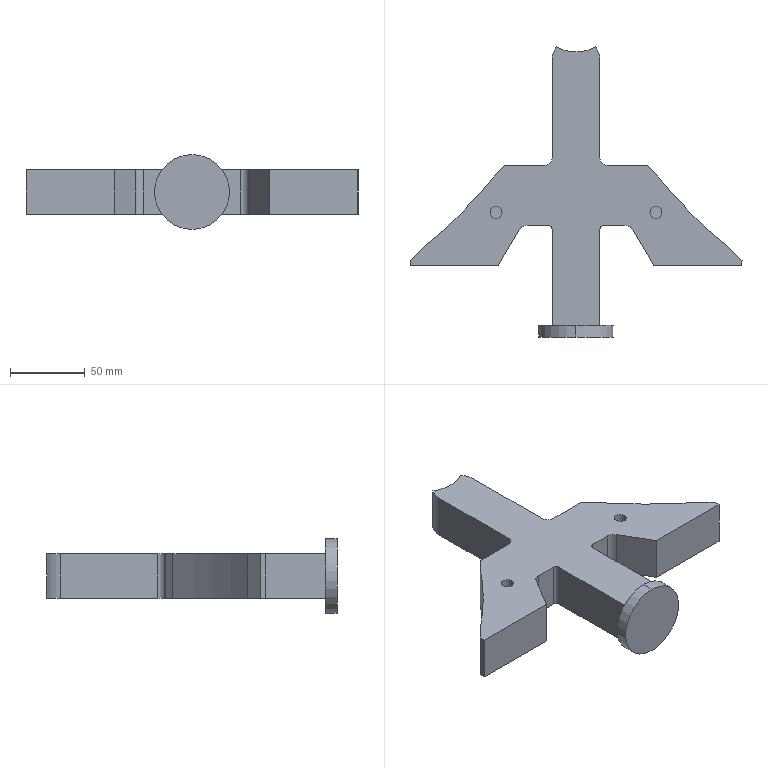Part | SolidWorks | features ICE 17, Cut 4, Chamfer 2, Extrusion 1, Fillet 1, MirrorPattern 1 | 1 solid | 41 faces | box 221.447 x 193.66 x 50 mm | volume 400373 mm3 | plane 24 | cylinder 15 | spline 2 | commonest cylinder face diameters 8 x4 5 x2 10 x2 12 x2 32 x2 50 x2